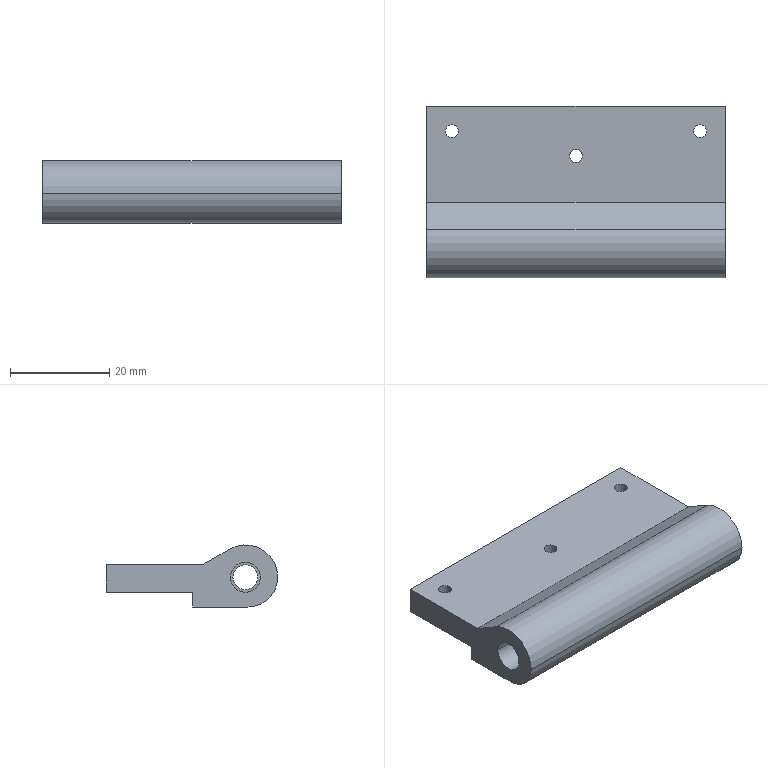NC program | NX | posted with a generic post | part box 60 x 34.5 x 12.5 mm
Whole program:
N10 G17 G21 G94 G90
(DRILLING_COPY_1_COPY , TOOL : D6A45)
N12 T07 M6
N14 G54
N16 G17 G0 G90 X28. Y-6. B0. C0. S3500 M3
N18 G43 Z30. H7
N20 G94 G81 G98 Z-1.8 F250. R3.
N22 G80
N24 G0 X28. Y-6. Z30.
N26 M5
(DRILLING_COPY_COPY_COPY_1_COPY , TOOL : 5.0ZT)
N28 T15 M6
N30 G54
N32 G17 G0 G90 X28. Y-6. B0. C0. S2000 M3
N34 G43 Z30. H15
N36 G94 G83 G98 Z-53.202 F100. Q2. R3.
N38 G80
N40 G0 X28. Y-6. Z30.
N42 M5
(HOLE_MILLING , TOOL : D4)
N44 T04 M6
N46 G54
N48 G17 G0 G90 X28. Y-6. B0. C0. S9500 M3
N50 G43 Z30. H4
N52 Z0.5
N54 G94 G3 X27.545 Y-5.545 R0.455 F1250.
N56 X27.09 Y-6. R0.455
N58 X27.09 Y-6. Z0.25 I0.91 J0.
N60 X27.09 Y-6. Z0. I0.91 J0.
N62 X27.09 Y-6. Z-0.25 I0.91 J0.
N64 X27.09 Y-6. Z-0.5 I0.91 J0.
N66 X27.09 Y-6. Z-0.75 I0.91 J0.
N68 X27.09 Y-6. Z-1. I0.91 J0.
N70 X27.09 Y-6. Z-1.25 I0.91 J0.
N72 X27.09 Y-6. Z-1.5 I0.91 J0.
N74 X27.09 Y-6. Z-1.75 I0.91 J0.
N76 X27.09 Y-6. Z-2. I0.91 J0.
N78 X27.09 Y-6. Z-2.25 I0.91 J0.
N80 X27.09 Y-6. Z-2.5 I0.91 J0.
N82 X27.09 Y-6. Z-2.75 I0.91 J0.
N84 X27.09 Y-6. Z-3. I0.91 J0.
N86 X27.09 Y-6. Z-3.25 I0.91 J0.
N88 X27.09 Y-6. Z-3.5 I0.91 J0.
N90 X27.09 Y-6. Z-3.75 I0.91 J0.
N92 X27.09 Y-6. Z-4. I0.91 J0.
N94 X27.09 Y-6. Z-4.25 I0.91 J0.
N96 X27.09 Y-6. Z-4.5 I0.91 J0.
N98 X27.09 Y-6. Z-4.75 I0.91 J0.
N100 X27.09 Y-6. Z-5. I0.91 J0.
N102 X27.09 Y-6. Z-5.25 I0.91 J0.
N104 X27.09 Y-6. Z-5.5 I0.91 J0.
N106 X27.09 Y-6. Z-5.75 I0.91 J0.
N108 X27.09 Y-6. Z-6. I0.91 J0.
N110 X27.09 Y-6. Z-6.25 I0.91 J0.
N112 X27.09 Y-6. Z-6.5 I0.91 J0.
N114 X27.09 Y-6. Z-6.75 I0.91 J0.
N116 X27.09 Y-6. Z-7. I0.91 J0.
N118 X27.09 Y-6. Z-7.25 I0.91 J0.
N120 X27.09 Y-6. Z-7.5 I0.91 J0.
N122 X27.09 Y-6. Z-7.75 I0.91 J0.
N124 X27.09 Y-6. Z-8. I0.91 J0.
N126 X27.09 Y-6. Z-8.25 I0.91 J0.
N128 X27.09 Y-6. Z-8.5 I0.91 J0.
N130 X27.09 Y-6. Z-8.75 I0.91 J0.
N132 X27.09 Y-6. Z-9. I0.91 J0.
N134 X27.09 Y-6. Z-9.25 I0.91 J0.
N136 X27.09 Y-6. Z-9.5 I0.91 J0.
N138 X27.09 Y-6. Z-9.75 I0.91 J0.
N140 X27.719 Y-6.865 Z-9.8 R0.91
N142 X28.865 Y-6.281 R0.91
N144 X27.719 Y-6.865 R-0.91
N146 X28.292 Y-6.573 R0.455
N148 X28. Y-6. R0.455
N150 G0 Z30.
N152 M5
(ZLEVEL_PROFILE_1_COPY_1_COPY_COPY_COPY_1_COPY_COPY_COPY_COPY_1 , TOOL : D6A45)
N154 T07 M6
N156 G54
N158 G17 G0 G90 X27.758 Y-6.816 B0. C0. S9500 M3
N160 G43 Z30. H7
N162 Z0.
N164 G94 G1 Z-1. F1000.
N166 X27.48 Y-7.751
N168 G3 X28. Y-8.051 R0.6
N170 X30.051 Y-6. R2.051
N172 X28. Y-8.051 R-2.051
N174 X28.52 Y-7.751 R0.6
N176 G1 X28.242 Y-6.816
N178 Z0.
N180 G0 Z30.
N182 M5
(CUTTERCOMP4 , TOOL : D4)
N184 T04 M6
N186 G54
N188 G17 G0 G90 X28. Y-6. B0. C0. S9500 M3
N190 G43 Z30. H4
N192 Z0.5
N194 G41 G94 G1 X27.997 Y-5.9 F1000. D4
N196 G3 X27.04 Y-6. R0.484
N198 X27.04 Y-6. Z-1.5 I0.96 J0.
N200 X27.04 Y-6. Z-3.5 I0.96 J0.
N202 X27.04 Y-6. Z-5.5 I0.96 J0.
N204 X27.04 Y-6. Z-7.5 I0.96 J0.
N206 X27.04 Y-6. Z-9.5 I0.96 J0.
N208 X27.436 Y-6.777 Z-9.8 R0.96
N210 X28.777 Y-6.564 R0.96
N212 X27.436 Y-6.777 R-0.96
N214 X28.079 Y-6.061 R0.484
N216 G40
N218 G1 X28. Y-6.
N220 G0 Z30.
N222 M5
N224 M2